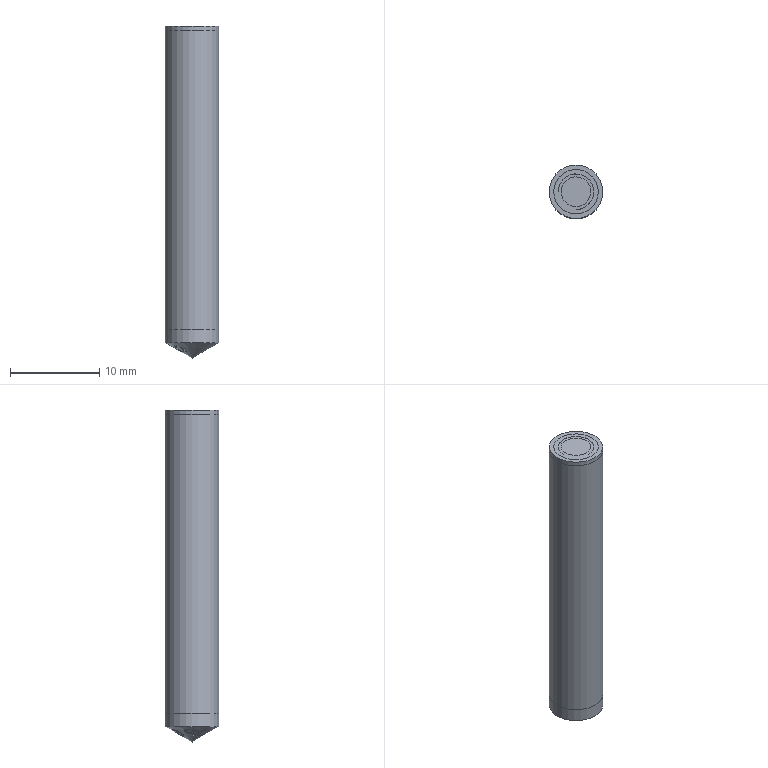Part | STEP file | EE030603500 | 2 solids | 45 faces | box 6 x 6 x 37.232 mm | volume 1919 mm3 | plane 15 | other 13 | cone 11 | cylinder 5 | torus 1 | commonest cylinder face diameters 6 x2 3.333 x1 3.987 x1 4 x1